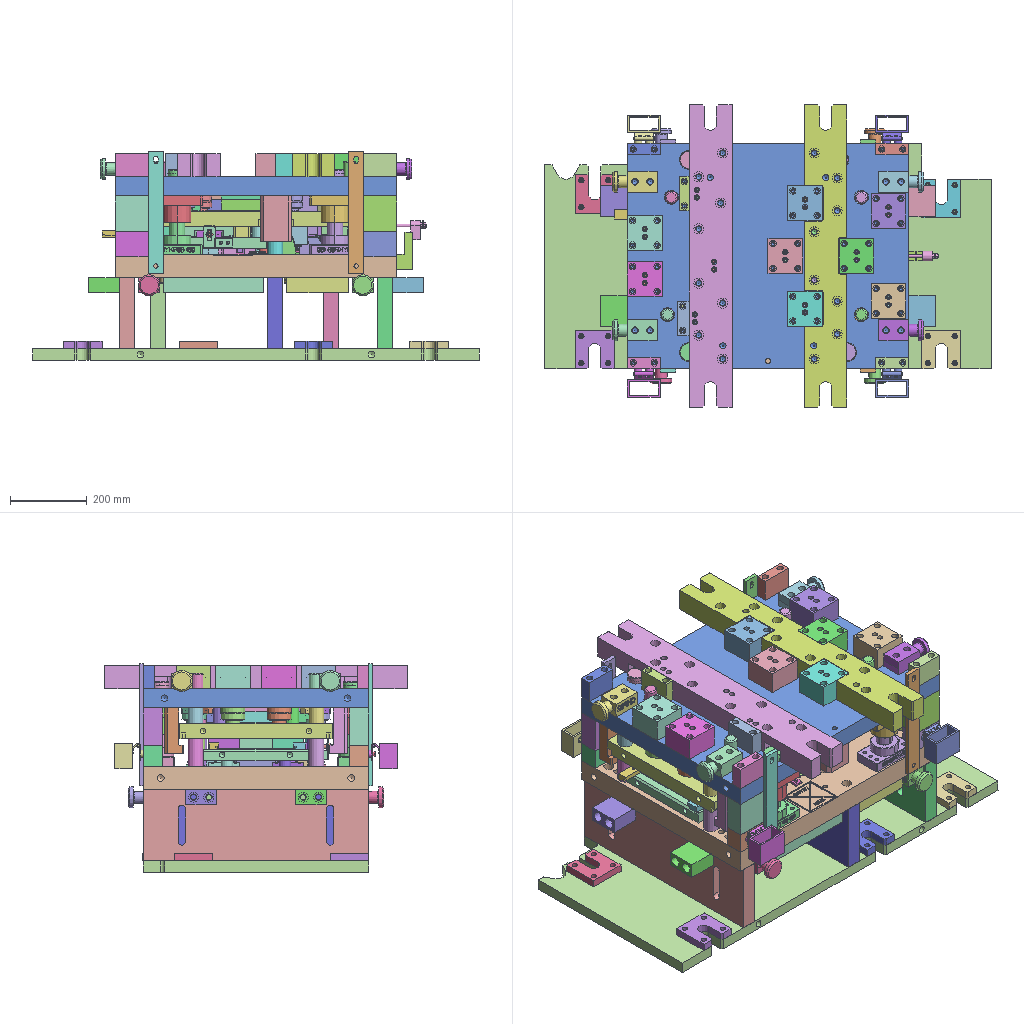Assembly | STEP file | 486 different items | 486 placed | box 1160 x 785 x 542 mm
Parts list (item | name | quantity | size | volume):
1 | 6-35_id1846_x_t | x1 | 8 x 8 x 38 mm | 1137 mm3
2 | 6-35_id1866_x_t | x1 | 8 x 8 x 38 mm | 1137 mm3
3 | - | x1 | 94 x 140 x 15 mm | 130830 mm3
4 | - | x1 | 58 x 85.001 x 56.5 mm | 200915 mm3
5 | - | x1 | 30 x 30 x 27 mm | 14276 mm3
6 | - | x1 | 30 x 30 x 27 mm | 14276 mm3
7 | - | x1 | 30 x 30 x 27 mm | 14276 mm3
8 | - | x1 | 60 x 80 x 56.5 mm | 99207 mm3
9 | - | x1 | 30 x 30 x 27 mm | 14276 mm3
10 | - | x1 | 40 x 40 x 72 mm | 79413 mm3
11 | - | x1 | 40 x 40 x 72 mm | 79413 mm3
12 | - | x1 | 40 x 40 x 72 mm | 79413 mm3
13 | - | x1 | 40 x 40 x 72 mm | 79413 mm3
14 | - | x1 | 99 x 140 x 30 mm | 280871 mm3
15 | - | x1 | 99 x 140 x 15 mm | 135777 mm3
16 | - | x1 | 40 x 40 x 72 mm | 79413 mm3
17 | - | x1 | 40 x 40 x 72 mm | 79413 mm3
18 | - | x1 | 42 x 25 x 98 mm | 60681 mm3
19 | - | x1 | 40 x 585 x 185 mm | 4078797 mm3
20 | - | x1 | 40 x 585 x 185 mm | 4012325 mm3
21 | - | x1 | 100 x 100 x 20 mm | 150755 mm3
22 | - | x1 | 100 x 100 x 20 mm | 150755 mm3
23 | - | x1 | 100 x 100 x 20 mm | 150755 mm3
24 | - | x1 | 40 x 255 x 185 mm | 1855337 mm3
25 | - | x1 | 40 x 255 x 185 mm | 1874377 mm3
26 | - | x1 | 40 x 585 x 185 mm | 4281820 mm3
27 | - | x1 | 85 x 50 x 55 mm | 210302 mm3
28 | - | x1 | 85 x 74 x 66.5 mm | 93814 mm3
29 | - | x1 | 63 x 73 x 30 mm | 93374 mm3
30 | - | x1 | 85 x 50 x 55 mm | 210302 mm3
31 | - | x1 | 85 x 74 x 66.5 mm | 93814 mm3
32 | - | x1 | 85 x 50 x 55 mm | 210302 mm3
33 | - | x1 | 85 x 74 x 66.5 mm | 93814 mm3
34 | - | x1 | 28 x 43 x 30 mm | 25680 mm3
35 | - | x1 | 85 x 50 x 55 mm | 210302 mm3
36 | - | x1 | 85 x 74 x 66.5 mm | 93814 mm3
37 | - | x1 | 19.1 x 19.1 x 30 mm | 8502 mm3
38 | - | x1 | 63 x 73 x 15 mm | 59595 mm3
39 | - | x1 | 30 x 30 x 15 mm | 8745 mm3
40 | - | x1 | 30 x 30 x 15 mm | 8745 mm3
41 | - | x1 | 30 x 30 x 15 mm | 8745 mm3
42 | - | x1 | 30 x 30 x 15 mm | 8745 mm3
43 | - | x1 | 30 x 30 x 15 mm | 8745 mm3
44 | - | x1 | 105 x 25 x 16 mm | 33608 mm3
45 | - | x1 | 45 x 25 x 16 mm | 13030 mm3
46 | - | x1 | 90 x 25 x 80 mm | 146448 mm3
47 | - | x1 | 90 x 25 x 80 mm | 146448 mm3
48 | - | x1 | 80 x 80 x 40 mm | 195367 mm3
49 | - | x1 | 80 x 80 x 40 mm | 195367 mm3
50 | - | x1 | 80 x 80 x 40 mm | 195367 mm3
51 | - | x1 | 80 x 80 x 40 mm | 195367 mm3
52 | - | x1 | 19.63 x 48.1 x 17 mm | 5552 mm3
53 | - | x1 | 75 x 27 x 53.7 mm | 8311 mm3
54 | - | x1 | 65 x 48 x 16 mm | 32002 mm3
55 | - | x1 | 15 x 70.5 x 16 mm | 11235 mm3
56 | - | x1 | 1160 x 585 x 30 mm | 18789042 mm3
57 | - | x1 | 100 x 100 x 20 mm | 150755 mm3
58 | - | x1 | 100 x 100 x 20 mm | 150755 mm3
59 | - | x1 | 260 x 40 x 40 mm | 385684 mm3
60 | - | x1 | - | 214873 mm3
61 | - | x1 | 260 x 40 x 40 mm | 385684 mm3
62 | - | x1 | 160 x 40 x 40 mm | 225684 mm3
63 | - | x1 | 160 x 40 x 40 mm | 225684 mm3
64 | - | x1 | 100 x 100 x 20 mm | 150755 mm3
65 | - | x1 | 40 x 10 x 317 mm | 124006 mm3
66 | - | x1 | 40 x 10 x 317 mm | 124006 mm3
67 | - | x1 | 40 x 10 x 317 mm | 124006 mm3
68 | - | x1 | 40 x 10 x 317 mm | 124006 mm3
69 | - | x1 | 58.148 x 85 x 56.5 mm | 200916 mm3
70 | - | x1 | 58 x 85 x 56.501 mm | 217515 mm3
71 | - | x1 | 40 x 55 x 53 mm | 73845 mm3
72 | - | x1 | 23.1 x 23.1 x 30 mm | 13334 mm3
73 | - | x1 | 65 x 75 x 45.001 mm | 106035 mm3
74 | - | x1 | 19 x 17 x 20 mm | 5075 mm3
75 | - | x1 | 15 x 13 x 20 mm | 2634 mm3
76 | - | x1 | 13.98 x 12 x 20 mm | 2357 mm3
77 | - | x1 | 70 x 120 x 30 mm | 188611 mm3
78 | - | x1 | 80 x 90 x 30 mm | 141495 mm3
79 | - | x1 | 80 x 90 x 15 mm | 69642 mm3
80 | - | x1 | 70 x 120 x 15 mm | 114867 mm3
81 | - | x1 | 40 x 55 x 53 mm | 73845 mm3
82 | - | x1 | 58 x 85 x 56.501 mm | 217785 mm3
83 | - | x1 | 58.914 x 80 x 15 mm | 42146 mm3
84 | - | x1 | 19.1 x 19.1 x 30 mm | 8502 mm3
85 | - | x1 | 60 x 80 x 56.5 mm | 99206 mm3
86 | - | x1 | 58.914 x 80 x 15 mm | 42146 mm3
87 | - | x1 | 105 x 25 x 16 mm | 33608 mm3
88 | - | x1 | 70 x 33 x 16 mm | 29565 mm3
89 | - | x1 | 20 x 25 x 7 mm | 3055 mm3
90 | - | x1 | 20 x 25 x 7 mm | 3055 mm3
91 | - | x1 | 20 x 25 x 7 mm | 3055 mm3
92 | - | x1 | 25 x 20 x 7 mm | 3055 mm3
93 | - | x1 | 730 x 585 x 60 mm | 23773121 mm3
94 | - | x1 | 240 x 52 x 30 mm | 250447 mm3
95 | - | x1 | 65 x 75 x 45.001 mm | 106042 mm3
96 | - | x1 | 19 x 17 x 20 mm | 5075 mm3
97 | - | x1 | 15 x 13 x 20 mm | 2634 mm3
98 | - | x1 | 13.98 x 12 x 20 mm | 2357 mm3
99 | - | x1 | 20 x 25 x 7 mm | 3055 mm3
100 | - | x1 | 26.045 x 93.231 x 17.45 mm | 4101 mm3
101 | - | x1 | 25 x 20 x 7 mm | 3055 mm3
102 | - | x1 | 94 x 140 x 30 mm | 271163 mm3
103 | - | x1 | 400 x 325 x 30 mm | 2323925 mm3
104 | CB-_id1534_x_t | x1 | 16 x 16 x 50 mm | 4584 mm3
105 | CB-_id1538_x_t | x1 | 16 x 16 x 50 mm | 4584 mm3
106 | CB-_id1554_x_t | x1 | 16 x 16 x 50 mm | 4584 mm3
107 | CB-_id1558_x_t | x1 | 16 x 16 x 50 mm | 4584 mm3
108 | CHP10_id1814_x_t | x1 | 118 x 55 x 55 mm | 202286 mm3
109 | CHP10_id1818_x_t | x1 | 118 x 55 x 55 mm | 202286 mm3
110 | CHP10_id1822_x_t | x1 | 118 x 55 x 55 mm | 202286 mm3
111 | CHP10_id1826_x_t | x1 | 118 x 55 x 55 mm | 202286 mm3
112 | CHP10_id1830_x_t | x1 | 55 x 118 x 55 mm | 202286 mm3
113 | CHP10_id1834_x_t | x1 | 55 x 118 x 55 mm | 202286 mm3
114 | CHP10_id1838_x_t | x1 | 55 x 118 x 55 mm | 202286 mm3
115 | CHP10_id1842_x_t | x1 | 55 x 118 x 55 mm | 202286 mm3
116 | D10-50_id1522_x_t | x1 | 10 x 10 x 50 mm | 3878 mm3
117 | D10-50_id1542_x_t | x1 | 10 x 10 x 50 mm | 3878 mm3
118 | D10-50_id1562_x_t | x1 | 10 x 10 x 50 mm | 3878 mm3
119 | D8-50_id106_x_t | x1 | 10 x 10 x 50 mm | 3919 mm3
120 | D8-50_id110_x_t | x1 | 10 x 10 x 50 mm | 3919 mm3
121 | D8-50_id114_x_t | x1 | 10 x 10 x 50 mm | 3919 mm3
122 | D8-50_id118_x_t | x1 | 10 x 10 x 50 mm | 3919 mm3
123 | D8-50_id1610_x_t | x1 | 8 x 8 x 30 mm | 1502 mm3
124 | D8-50_id1618_x_t | x1 | 8 x 8 x 30 mm | 1502 mm3
125 | D8-50_id162_x_t | x1 | 8 x 8 x 45 mm | 2256 mm3
126 | D8-50_id1630_x_t | x1 | 8 x 8 x 30 mm | 1502 mm3
127 | D8-50_id1638_x_t | x1 | 8 x 8 x 30 mm | 1502 mm3
128 | D8-50_id1650_x_t | x1 | 8 x 8 x 30 mm | 1502 mm3
129 | D8-50_id1654_x_t | x1 | 8 x 8 x 30 mm | 1502 mm3
130 | D8-50_id1658_x_t | x1 | 8 x 8 x 30 mm | 1502 mm3
131 | D8-50_id166_x_t | x1 | 8 x 8 x 45 mm | 2256 mm3
132 | D8-50_id1670_x_t | x1 | 8 x 8 x 30 mm | 1502 mm3
133 | D8-50_id1682_x_t | x1 | 8 x 8 x 30 mm | 1502 mm3
134 | D8-50_id1686_x_t | x1 | 8 x 8 x 30 mm | 1502 mm3
135 | D8-50_id290_x_t | x1 | 8 x 8 x 30 mm | 1502 mm3
136 | D8-50_id294_x_t | x1 | 8 x 8 x 30 mm | 1502 mm3
137 | D8-50_id350_x_t | x1 | 8 x 8 x 45 mm | 2256 mm3
138 | D8-50_id358_x_t | x1 | 8 x 8 x 45 mm | 2256 mm3
139 | D8-50_id390_x_t | x1 | 8 x 8 x 30 mm | 1502 mm3
140 | D8-50_id394_x_t | x1 | 8 x 8 x 30 mm | 1502 mm3
141 | D8-50_id402_x_t | x1 | 10 x 10 x 40 mm | 3134 mm3
142 | D8-50_id406_x_t | x1 | 8 x 8 x 30 mm | 1502 mm3
143 | D8-50_id422_x_t | x1 | 8 x 8 x 30 mm | 1502 mm3
144 | D8-50_id442_x_t | x1 | 10 x 10 x 40 mm | 3134 mm3
145 | D8-50_id470_x_t | x1 | 8 x 8 x 30 mm | 1502 mm3
146 | D8-50_id474_x_t | x1 | 8 x 8 x 30 mm | 1502 mm3
147 | D8-50_id482_x_t | x1 | 8 x 8 x 30 mm | 1502 mm3
148 | D8-50_id486_x_t | x1 | 8 x 8 x 30 mm | 1502 mm3
149 | D8-50_id50_x_t | x1 | 10 x 10 x 50 mm | 3919 mm3
150 | D8-50_id58_x_t | x1 | 10 x 10 x 50 mm | 3919 mm3
151 | D8-50_id618_x_t | x1 | 8 x 8 x 30 mm | 1502 mm3
152 | D8-50_id622_x_t | x1 | 8 x 8 x 30 mm | 1502 mm3
153 | D8-50_id78_x_t | x1 | 10 x 10 x 40 mm | 3134 mm3
154 | D8-50_id82_x_t | x1 | 10 x 10 x 40 mm | 3134 mm3
155 | GSV170-7_id1154_x_t | x1 | 50 x 50 x 114 mm | 158224 mm3
156 | GSV170-7_id1158_x_t | x1 | 50 x 50 x 114 mm | 158224 mm3
157 | GSV170-7_id1162_x_t | x1 | 50 x 50 x 114 mm | 158224 mm3
158 | GSV170-7_id1166_x_t | x1 | 50 x 50 x 114 mm | 158224 mm3
159 | GSV170-7_id1170_x_t | x1 | 50 x 50 x 114 mm | 158224 mm3
160 | GSV170-7_id1174_x_t | x1 | 50 x 50 x 114 mm | 158224 mm3
161 | GSV170-7_id1178_x_t | x1 | 63 x 63 x 120 mm | 273871 mm3
162 | GSV170-7_id1182_x_t | x1 | 63 x 63 x 120 mm | 273871 mm3
163 | GSV170-7_id1186_x_t | x1 | 63 x 63 x 120 mm | 273871 mm3
164 | GSV170-7_id1190_x_t | x1 | 63 x 63 x 120 mm | 273871 mm3
165 | GSV170-7_id1266_x_t | x1 | 50 x 50 x 114 mm | 158224 mm3
166 | GSV170-7_id502_x_t | x1 | 19 x 19 x 106 mm | 21365 mm3
167 | GSV170-7_id510_x_t | x1 | 19 x 19 x 106 mm | 21365 mm3
168 | GSV170-7_id526_x_t | x1 | 19 x 19 x 106 mm | 21365 mm3
169 | GSV170-7_id546_x_t | x1 | 19 x 19 x 106 mm | 21365 mm3
170 | GSV170-7_id666_x_t | x1 | 19 x 19 x 106 mm | 21365 mm3
171 | GSV170-7_id730_x_t | x1 | 19 x 19 x 106 mm | 21365 mm3
172 | LPS 2-10_id1006_x_t | x1 | 8 x 8 x 60 mm | 2567 mm3
173 | LPS 2-10_id1010_x_t | x1 | 8 x 8 x 60 mm | 2567 mm3
174 | LPS 2-10_id1014_x_t | x1 | 8 x 8 x 60 mm | 2567 mm3
175 | LPS 2-10_id1038_x_t | x1 | 8 x 8 x 60 mm | 2567 mm3
176 | LPS 2-10_id1042_x_t | x1 | 8 x 8 x 60 mm | 2567 mm3
177 | LPS 2-10_id1046_x_t | x1 | 8 x 8 x 60 mm | 2567 mm3
178 | LPS 2-10_id1050_x_t | x1 | 8 x 8 x 60 mm | 2567 mm3
179 | LPS 2-10_id898_x_t | x1 | 8 x 8 x 60 mm | 2567 mm3
180 | LPS 2-10_id902_x_t | x1 | 8 x 8 x 60 mm | 2567 mm3
181 | LPS 2-10_id906_x_t | x1 | 8 x 8 x 60 mm | 2567 mm3
182 | LPS 2-10_id910_x_t | x1 | 8 x 8 x 60 mm | 2567 mm3
183 | LPS 2-10_id914_x_t | x1 | 8 x 8 x 60 mm | 2567 mm3
184 | LPS 2-10_id918_x_t | x1 | 8 x 8 x 60 mm | 2567 mm3
185 | LPS 2-10_id922_x_t | x1 | 8 x 8 x 60 mm | 2567 mm3
186 | LPS 2-10_id926_x_t | x1 | 8 x 8 x 60 mm | 2567 mm3
187 | LPS 2-10_id930_x_t | x1 | 8 x 8 x 60 mm | 2567 mm3
188 | LPS 2-10_id934_x_t | x1 | 8 x 8 x 60 mm | 2567 mm3
189 | LPS 2-10_id938_x_t | x1 | 8 x 8 x 60 mm | 2567 mm3
190 | LPS 2-10_id942_x_t | x1 | 8 x 8 x 60 mm | 2567 mm3
191 | LPS 2-10_id946_x_t | x1 | 8 x 8 x 60 mm | 2567 mm3
192 | LPS 2-10_id950_x_t | x1 | 8 x 8 x 60 mm | 2567 mm3
193 | LPS 2-10_id954_x_t | x1 | 8 x 8 x 60 mm | 2567 mm3
194 | LPS 2-10_id974_x_t | x1 | 8 x 8 x 60 mm | 2567 mm3
195 | LPS 2-10_id978_x_t | x1 | 8 x 8 x 60 mm | 2567 mm3
196 | LPS 2-10_id982_x_t | x1 | 8 x 8 x 60 mm | 2567 mm3
197 | LPS 2-10_id986_x_t | x1 | 8 x 8 x 60 mm | 2567 mm3
198 | LPS 2-10_id990_x_t | x1 | 8 x 8 x 60 mm | 2567 mm3
199 | LPS 2-10_id994_x_t | x1 | 8 x 8 x 60 mm | 2567 mm3
200 | LPS 2-10_id998_x_t | x1 | 8 x 8 x 60 mm | 2567 mm3
201 | M3-10_id130_x_t | x1 | 16 x 16 x 55 mm | 4808 mm3
202 | M3-10_id134_x_t | x1 | 16 x 16 x 55 mm | 4808 mm3
203 | M3-10_id1366_x_t | x1 | 43 x 13 x 13 mm | 2482 mm3
204 | M3-10_id1414_x_t | x1 | 16 x 16 x 45 mm | 4022 mm3
205 | M3-10_id1418_x_t | x1 | 16 x 16 x 45 mm | 4022 mm3
206 | M3-10_id1422_x_t | x1 | 13 x 33 x 13 mm | 1987 mm3
207 | M3-10_id1426_x_t | x1 | 13 x 33 x 13 mm | 1987 mm3
208 | M3-10_id1434_x_t | x1 | 16 x 16 x 45 mm | 4022 mm3
209 | M3-10_id1438_x_t | x1 | 13 x 33 x 13 mm | 1987 mm3
210 | M3-10_id1442_x_t | x1 | 13 x 33 x 13 mm | 1987 mm3
211 | M3-10_id1454_x_t | x1 | 16 x 16 x 45 mm | 4022 mm3
212 | M3-10_id1474_x_t | x1 | 16 x 16 x 45 mm | 4022 mm3
213 | M3-10_id1486_x_t | x1 | 16 x 16 x 45 mm | 4022 mm3
214 | M3-10_id154_x_t | x1 | 13 x 13 x 48 mm | 2734 mm3
215 | M3-10_id1570_x_t | x1 | 13 x 13 x 28 mm | 1728 mm3
216 | M3-10_id1578_x_t | x1 | 13 x 13 x 28 mm | 1728 mm3
217 | M3-10_id1582_x_t | x1 | 13 x 13 x 28 mm | 1728 mm3
218 | M3-10_id158_x_t | x1 | 13 x 13 x 48 mm | 2734 mm3
219 | M3-10_id1594_x_t | x1 | 13 x 13 x 28 mm | 1728 mm3
220 | M3-10_id1602_x_t | x1 | 13 x 13 x 28 mm | 1728 mm3
221 | M3-10_id1614_x_t | x1 | 13 x 13 x 28 mm | 1742 mm3
222 | M3-10_id1622_x_t | x1 | 13 x 13 x 28 mm | 1742 mm3
223 | M3-10_id1634_x_t | x1 | 13 x 13 x 28 mm | 1742 mm3
224 | M3-10_id1646_x_t | x1 | 13 x 13 x 48 mm | 2734 mm3
225 | M3-10_id1662_x_t | x1 | 13 x 13 x 48 mm | 2734 mm3
226 | M3-10_id1674_x_t | x1 | 13 x 13 x 28 mm | 1742 mm3
227 | M3-10_id1678_x_t | x1 | 13 x 13 x 28 mm | 1742 mm3
228 | M3-10_id206_x_t | x1 | 20 x 8.5 x 8.5 mm | 482.387 mm3
229 | M3-10_id210_x_t | x1 | 20 x 8.5 x 8.5 mm | 482.387 mm3
230 | M3-10_id214_x_t | x1 | 16 x 16 x 40 mm | 3630 mm3
231 | M3-10_id218_x_t | x1 | 16 x 16 x 40 mm | 3630 mm3
232 | M3-10_id222_x_t | x1 | 16 x 16 x 40 mm | 3630 mm3
233 | M3-10_id226_x_t | x1 | 16 x 16 x 40 mm | 3630 mm3
234 | M3-10_id234_x_t | x1 | 16 x 16 x 40 mm | 3630 mm3
235 | M3-10_id238_x_t | x1 | 16 x 16 x 40 mm | 3630 mm3
236 | M3-10_id258_x_t | x1 | 8.5 x 8.5 x 20 mm | 456.375 mm3
237 | M3-10_id262_x_t | x1 | 8.5 x 8.5 x 20 mm | 456.375 mm3
238 | M3-10_id266_x_t | x1 | 8.5 x 8.5 x 20 mm | 456.375 mm3
239 | M3-10_id274_x_t | x1 | 10 x 10 x 46 mm | 1459 mm3
240 | M3-10_id278_x_t | x1 | 13 x 13 x 33 mm | 1980 mm3
241 | M3-10_id282_x_t | x1 | 13 x 13 x 33 mm | 1980 mm3
242 | M3-10_id286_x_t | x1 | 13 x 13 x 33 mm | 1980 mm3
243 | M3-10_id302_x_t | x1 | 20 x 8.5 x 8.5 mm | 482.387 mm3
244 | M3-10_id306_x_t | x1 | 16 x 16 x 40 mm | 3630 mm3
245 | M3-10_id310_x_t | x1 | 16 x 16 x 40 mm | 3630 mm3
246 | M3-10_id314_x_t | x1 | 20 x 8.5 x 8.5 mm | 482.387 mm3
247 | M3-10_id318_x_t | x1 | 16 x 16 x 40 mm | 3630 mm3
248 | M3-10_id322_x_t | x1 | 16 x 16 x 40 mm | 3630 mm3
249 | M3-10_id334_x_t | x1 | 16 x 16 x 40 mm | 3630 mm3
250 | M3-10_id342_x_t | x1 | 16 x 16 x 40 mm | 3630 mm3
251 | M3-10_id346_x_t | x1 | 13 x 13 x 48 mm | 2734 mm3
252 | M3-10_id34_x_t | x1 | 8.5 x 8.5 x 20 mm | 456.375 mm3
253 | M3-10_id354_x_t | x1 | 13 x 13 x 48 mm | 2734 mm3
254 | M3-10_id370_x_t | x1 | 8.5 x 8.5 x 20 mm | 456.375 mm3
255 | M3-10_id374_x_t | x1 | 13 x 13 x 28 mm | 1728 mm3
256 | M3-10_id378_x_t | x1 | 13 x 13 x 28 mm | 1728 mm3
257 | M3-10_id382_x_t | x1 | 13 x 13 x 28 mm | 1728 mm3
258 | M3-10_id386_x_t | x1 | 13 x 13 x 28 mm | 1728 mm3
259 | M3-10_id38_x_t | x1 | 8.5 x 8.5 x 20 mm | 456.375 mm3
260 | M3-10_id398_x_t | x1 | 13 x 13 x 28 mm | 1728 mm3
261 | M3-10_id410_x_t | x1 | 13 x 13 x 33 mm | 1980 mm3
262 | M3-10_id414_x_t | x1 | 13 x 13 x 33 mm | 1980 mm3
263 | M3-10_id418_x_t | x1 | 13 x 13 x 28 mm | 1728 mm3
264 | M3-10_id42_x_t | x1 | 16 x 16 x 55 mm | 4808 mm3
265 | M3-10_id430_x_t | x1 | 13 x 13 x 33 mm | 1980 mm3
266 | M3-10_id438_x_t | x1 | 13 x 13 x 28 mm | 1728 mm3
267 | M3-10_id446_x_t | x1 | 13 x 13 x 28 mm | 1728 mm3
268 | M3-10_id450_x_t | x1 | 13 x 13 x 33 mm | 1980 mm3
269 | M3-10_id462_x_t | x1 | 13 x 13 x 28 mm | 1742 mm3
270 | M3-10_id466_x_t | x1 | 13 x 13 x 28 mm | 1742 mm3
271 | M3-10_id46_x_t | x1 | 16 x 16 x 55 mm | 4808 mm3
272 | M3-10_id478_x_t | x1 | 13 x 13 x 28 mm | 1742 mm3
273 | M3-10_id54_x_t | x1 | 16 x 16 x 55 mm | 4808 mm3
274 | M3-10_id562_x_t | x1 | 10 x 10 x 26 mm | 877.848 mm3
275 | M3-10_id566_x_t | x1 | 10 x 10 x 26 mm | 877.848 mm3
276 | M3-10_id570_x_t | x1 | 10 x 10 x 26 mm | 877.848 mm3
277 | M3-10_id574_x_t | x1 | 10 x 10 x 26 mm | 877.848 mm3
278 | M3-10_id578_x_t | x1 | 10 x 10 x 26 mm | 877.848 mm3
279 | M3-10_id582_x_t | x1 | 10 x 10 x 26 mm | 877.848 mm3
280 | M3-10_id586_x_t | x1 | 10 x 10 x 26 mm | 877.848 mm3
281 | M3-10_id590_x_t | x1 | 10 x 10 x 26 mm | 877.848 mm3
282 | M3-10_id594_x_t | x1 | 13 x 13 x 28 mm | 1756 mm3
283 | M3-10_id598_x_t | x1 | 13 x 13 x 28 mm | 1756 mm3
284 | M3-10_id602_x_t | x1 | 13 x 13 x 28 mm | 1756 mm3
285 | M3-10_id610_x_t | x1 | 8.5 x 8.5 x 20 mm | 456.375 mm3
286 | M3-10_id626_x_t | x1 | 13 x 13 x 33 mm | 1980 mm3
287 | M3-10_id62_x_t | x1 | 13 x 13 x 33 mm | 1980 mm3
288 | M3-10_id630_x_t | x1 | 8.5 x 8.5 x 20 mm | 456.375 mm3
289 | M3-10_id634_x_t | x1 | 8.5 x 8.5 x 20 mm | 456.375 mm3
290 | M3-10_id642_x_t | x1 | 13 x 13 x 33 mm | 1980 mm3
291 | M3-10_id654_x_t | x1 | 13 x 13 x 33 mm | 1980 mm3
292 | M3-10_id658_x_t | x1 | 10 x 10 x 26 mm | 877.848 mm3
293 | M3-10_id662_x_t | x1 | 10 x 10 x 26 mm | 877.848 mm3
294 | M3-10_id66_x_t | x1 | 13 x 13 x 33 mm | 1980 mm3
295 | M3-10_id674_x_t | x1 | 13 x 13 x 33 mm | 1980 mm3
296 | M3-10_id678_x_t | x1 | 13 x 13 x 33 mm | 1980 mm3
297 | M3-10_id682_x_t | x1 | 13 x 13 x 33 mm | 1980 mm3
298 | M3-10_id686_x_t | x1 | 13 x 13 x 33 mm | 1980 mm3
299 | M3-10_id694_x_t | x1 | 13 x 13 x 33 mm | 1980 mm3
300 | M3-10_id702_x_t | x1 | 13 x 13 x 28 mm | 1756 mm3
301 | M3-10_id706_x_t | x1 | 10 x 10 x 26 mm | 877.848 mm3
302 | M3-10_id70_x_t | x1 | 13 x 13 x 33 mm | 1980 mm3
303 | M3-10_id710_x_t | x1 | 10 x 10 x 26 mm | 877.848 mm3
304 | M3-10_id714_x_t | x1 | 13 x 13 x 28 mm | 1756 mm3
305 | M3-10_id738_x_t | x1 | 13 x 13 x 33 mm | 1980 mm3
306 | M3-10_id74_x_t | x1 | 13 x 13 x 33 mm | 1980 mm3
307 | M3-10_id94_x_t | x1 | 16 x 16 x 55 mm | 4808 mm3
308 | M3-10_id98_x_t | x1 | 16 x 16 x 55 mm | 4808 mm3
309 | M6-40_id1082_x_t | x1 | 16 x 16 x 40 mm | 3648 mm3
310 | M6-40_id1090_x_t | x1 | 16 x 16 x 40 mm | 3648 mm3
311 | M6-40_id1098_x_t | x1 | 16 x 16 x 40 mm | 3648 mm3
312 | M6-40_id1106_x_t | x1 | 16 x 16 x 40 mm | 3648 mm3
313 | M6-40_id1114_x_t | x1 | 16 x 16 x 70 mm | 6004 mm3
314 | M6-40_id1122_x_t | x1 | 16 x 16 x 70 mm | 6004 mm3
315 | M6-40_id1126_x_t | x1 | 16 x 16 x 70 mm | 6004 mm3
316 | M6-40_id1130_x_t | x1 | 16 x 16 x 70 mm | 6004 mm3
317 | M6-40_id1138_x_t | x1 | 16 x 16 x 70 mm | 6004 mm3
318 | M6-40_id1146_x_t | x1 | 16 x 16 x 70 mm | 6004 mm3
319 | MSW12-10_id1850_x_t | x1 | 12.005 x 12.005 x 10 mm | 1118 mm3
320 | MSW12-10_id1862_x_t | x1 | 12.005 x 12.005 x 10 mm | 1118 mm3
321 | PN_0001_id1150_x_t | x1 | 730 x 585 x 50 mm | 18693036 mm3
322 | PN_0002_id1798_x_t | x1 | 85 x 30 x 60 mm | 133679 mm3
323 | PN_0002_id1802_x_t | x1 | 85 x 30 x 60 mm | 133679 mm3
324 | PN_0002_id1806_x_t | x1 | 85 x 30 x 60 mm | 133679 mm3
325 | PN_0002_id1810_x_t | x1 | 85 x 30 x 60 mm | 133679 mm3
326 | PN_0003_id1490_x_t | x1 | 90 x 90 x 60 mm | 430512 mm3
327 | PN_0003_id1494_x_t | x1 | 90 x 90 x 60 mm | 430512 mm3
328 | PN_0004_id1502_x_t | x1 | 30 x 90 x 60 mm | 142679 mm3
329 | PN_0005_id1498_x_t | x1 | 25 x 90 x 60 mm | 115679 mm3
330 | PN_0006_id1766_x_t | x1 | 112 x 785 x 60 mm | 4657225 mm3
331 | PN_0007_id1774_x_t | x1 | 90 x 90 x 60 mm | 428886 mm3
332 | PN_0007_id1778_x_t | x1 | 90 x 90 x 60 mm | 428886 mm3
333 | PN_0007_id1782_x_t | x1 | 90 x 90 x 60 mm | 428886 mm3
334 | PN_0007_id1786_x_t | x1 | 90 x 90 x 60 mm | 428886 mm3
335 | PN_0007_id1790_x_t | x1 | 90 x 90 x 60 mm | 428886 mm3
336 | PN_0007_id1794_x_t | x1 | 90 x 90 x 60 mm | 428886 mm3
337 | PN_0008_id1770_x_t | x1 | 110 x 785 x 60 mm | 3912002 mm3
338 | PN_0009_id1210_x_t | x1 | 40 x 40 x 40 mm | 44485 mm3
339 | PN_0009_id1214_x_t | x1 | 40 x 40 x 40 mm | 44485 mm3
340 | PN_0009_id1218_x_t | x1 | 40 x 40 x 40 mm | 44485 mm3
341 | PN_0009_id1222_x_t | x1 | 40 x 40 x 40 mm | 44485 mm3
342 | PN_0009_id1226_x_t | x1 | 40 x 40 x 40 mm | 44485 mm3
343 | PN_0009_id1230_x_t | x1 | 40 x 40 x 40 mm | 44485 mm3
344 | PN_0009_id1234_x_t | x1 | 40 x 40 x 40 mm | 44485 mm3
345 | PN_0009_id1238_x_t | x1 | 40 x 40 x 40 mm | 44485 mm3
346 | PN_0009_id1242_x_t | x1 | 40 x 40 x 40 mm | 44485 mm3
347 | PN_0009_id1246_x_t | x1 | 40 x 40 x 40 mm | 44485 mm3
348 | PN_0009_id1250_x_t | x1 | 40 x 40 x 40 mm | 44485 mm3
349 | PN_0009_id1254_x_t | x1 | 40 x 40 x 40 mm | 44485 mm3
350 | PN_0009_id1258_x_t | x1 | 40 x 40 x 40 mm | 44485 mm3
351 | PN_0009_id1262_x_t | x1 | 40 x 40 x 40 mm | 44485 mm3
352 | PN_0009_id1294_x_t | x1 | 40 x 40 x 40 mm | 44485 mm3
353 | PN_0009_id1302_x_t | x1 | 40 x 40 x 40 mm | 44485 mm3
354 | PN_0010_id1734_x_t | x1 | 30.406 x 30.406 x 15 mm | 5664 mm3
355 | PN_0010_id1738_x_t | x1 | 30.406 x 30.406 x 15 mm | 5664 mm3
356 | PN_0010_id1742_x_t | x1 | 28.807 x 23.857 x 15 mm | 5664 mm3
357 | PN_0010_id1746_x_t | x1 | 28.807 x 23.857 x 15 mm | 5664 mm3
358 | PN_0010_id1750_x_t | x1 | 27.746 x 22.068 x 15 mm | 5664 mm3
359 | PN_0010_id1754_x_t | x1 | 27.746 x 22.068 x 15 mm | 5664 mm3
360 | PN_0010_id1758_x_t | x1 | 29.858 x 30.721 x 15 mm | 5664 mm3
361 | PN_0010_id1762_x_t | x1 | 29.858 x 30.721 x 15 mm | 5664 mm3
362 | PN_0011_id1938_x_t | x1 | 30 x 16 x 16 mm | 6162 mm3
363 | PN_0012_id1934_x_t | x1 | 30 x 16 x 16 mm | 6162 mm3
364 | PN_0013_id878_x_t | x1 | 25 x 40 x 50 mm | 37635 mm3
365 | PN_0014_id874_x_t | x1 | 25 x 40 x 50 mm | 37635 mm3
366 | PN_0015_id866_x_t | x1 | 95 x 130 x 28 mm | 241686 mm3
367 | PN_0016_id882_x_t | x1 | 40 x 25 x 50 mm | 37460 mm3
368 | PN_0017_id886_x_t | x1 | 90 x 75 x 28 mm | 120807 mm3
369 | PN_0018_id894_x_t | x1 | 43 x 30 x 50 mm | 41594 mm3
370 | PN_0019_id962_x_t | x1 | 105 x 120 x 28 mm | 217134 mm3
371 | PN_0020_id958_x_t | x1 | 105 x 120 x 28 mm | 217134 mm3
372 | PN_0021_id1034_x_t | x1 | 51 x 55 x 50 mm | 79399 mm3
373 | PN_0022_id1018_x_t | x1 | 105 x 176 x 28 mm | 281247 mm3
374 | PN_0023_id1002_x_t | x1 | 51 x 55 x 50 mm | 79567 mm3
375 | PN_0024_id1030_x_t | x1 | 60 x 85 x 28 mm | 85179 mm3
376 | PN_0025_id842_x_t | x1 | 727.5 x 395 x 40 mm | 9281090 mm3
377 | PN_0026_id138_x_t | x1 | 15 x 17 x 108 mm | 21787 mm3
378 | PN_0027_id762_x_t | x1 | 48.641 x 98 x 108 mm | 278629 mm3
379 | PN_0028_id758_x_t | x1 | 48.641 x 98 x 108 mm | 278628 mm3
380 | PN_0029_id850_x_t | x1 | 51.676 x 85.003 x 65 mm | 145640 mm3
381 | PN_0030_id186_x_t | x1 | 51.676 x 85 x 65 mm | 145641 mm3
382 | PN_0031_id862_x_t | x1 | 42.5 x 42 x 101 mm | 91343 mm3
383 | PN_0032_id1054_x_t | x1 | 63.914 x 80 x 35 mm | 137778 mm3
384 | PN_0033_id754_x_t | x1 | 63.914 x 80 x 35 mm | 137778 mm3
385 | PN_0034_id750_x_t | x1 | 290 x 208 x 25 mm | 1200557 mm3
386 | PN_0035_id190_x_t | x1 | 50.466 x 210 x 37 mm | 295873 mm3
387 | PN_0036_id230_x_t | x1 | 149.23 x 42 x 25 mm | 138214 mm3
388 | PN_0037_id1074_x_t | x1 | 70 x 85 x 53 mm | 208410 mm3
389 | PN_0038_id1942_x_t | x1 | 70 x 85 x 53 mm | 208411 mm3
390 | PN_0039_id846_x_t | x1 | 115 x 175 x 25 mm | 409284 mm3
391 | PN_0040_id1406_x_t | x1 | 85 x 50 x 97 mm | 372174 mm3
392 | PN_0040_id1446_x_t | x1 | 85 x 50 x 97 mm | 372174 mm3
393 | PN_0040_id1462_x_t | x1 | 85 x 50 x 97 mm | 372174 mm3
394 | PN_0040_id1478_x_t | x1 | 85 x 50 x 97 mm | 372174 mm3
395 | PN_0041_id1270_x_t | x1 | 80 x 50 x 118 mm | 264145 mm3
396 | PN_0041_id1274_x_t | x1 | 80 x 50 x 118 mm | 264145 mm3
397 | PN_0041_id1278_x_t | x1 | 80 x 50 x 118 mm | 264145 mm3
398 | PN_0041_id1282_x_t | x1 | 80 x 50 x 118 mm | 264145 mm3
399 | PN_0041_id1286_x_t | x1 | 80 x 50 x 118 mm | 264145 mm3
400 | PN_0041_id1290_x_t | x1 | 80 x 50 x 118 mm | 264145 mm3
401 | PN_0042_id870_x_t | x1 | 95 x 130 x 10 mm | 115889 mm3
402 | PN_0043_id890_x_t | x1 | 90 x 75 x 10 mm | 57234 mm3
403 | PN_0044_id966_x_t | x1 | 105 x 120 x 10 mm | 118397 mm3
404 | PN_0044_id970_x_t | x1 | 105 x 120 x 10 mm | 118397 mm3
405 | PN_0045_id858_x_t | x1 | 74.676 x 85 x 110 mm | 490058 mm3
406 | PN_0046_id854_x_t | x1 | 74.676 x 85 x 110 mm | 490062 mm3
407 | PN_0047_id1022_x_t | x1 | 105 x 176 x 10 mm | 142706 mm3
408 | PN_0048_id1026_x_t | x1 | 60 x 85 x 10 mm | 42512 mm3
409 | PN_0049_id1058_x_t | x1 | 13 x 13 x 100 mm | 5213 mm3
410 | PN_0049_id1062_x_t | x1 | 13 x 13 x 100 mm | 5213 mm3
411 | PN_0050_id1066_x_t | x1 | 15 x 15 x 100 mm | 8031 mm3
412 | PN_0051_id1710_x_t | x1 | 13 x 13 x 100 mm | 4994 mm3
413 | PN_0051_id1714_x_t | x1 | 13 x 13 x 100 mm | 4994 mm3
414 | PN_0052_id1718_x_t | x1 | 15 x 15 x 100 mm | 7737 mm3
415 | PN_0052_id1722_x_t | x1 | 15 x 15 x 100 mm | 7737 mm3
416 | PN_0053_id1726_x_t | x1 | 15 x 11.5 x 100 mm | 7176 mm3
417 | PN_0053_id1730_x_t | x1 | 15 x 11.5 x 100 mm | 7176 mm3
418 | PN_0054_id498_x_t | x1 | 45 x 25 x 9.2 mm | 6185 mm3
419 | PN_0054_id518_x_t | x1 | 45 x 25 x 9.2 mm | 6185 mm3
420 | PN_0054_id534_x_t | x1 | 45 x 25 x 9.2 mm | 6185 mm3
421 | PN_0054_id554_x_t | x1 | 45 x 25 x 9.2 mm | 6185 mm3
422 | PN_0054_id670_x_t | x1 | 25 x 45 x 9.2 mm | 6185 mm3
423 | PN_0054_id722_x_t | x1 | 25 x 45 x 9.2 mm | 6185 mm3
424 | PN_0055_id1202_x_t | x1 | 42 x 42 x 40 mm | 22994 mm3
425 | PN_0055_id1322_x_t | x1 | 42 x 42 x 40 mm | 22995 mm3
426 | PN_0055_id1330_x_t | x1 | 42 x 42 x 40 mm | 22994 mm3
427 | PN_0055_id1354_x_t | x1 | 42 x 42 x 40 mm | 22995 mm3
428 | PN_0056_id1706_x_t | x1 | 16 x 16 x 45 mm | 3853 mm3
429 | PN_0057_id1194_x_t | x1 | 44 x 44 x 153 mm | 127630 mm3
430 | PN_0057_id1198_x_t | x1 | 16 x 16 x 40 mm | 4064 mm3
431 | PN_0057_id1206_x_t | x1 | 40 x 40 x 16 mm | 13382 mm3
432 | PN_0057_id1310_x_t | x1 | 44 x 44 x 153 mm | 127629 mm3
433 | PN_0057_id1314_x_t | x1 | 40 x 40 x 16 mm | 13382 mm3
434 | PN_0057_id1318_x_t | x1 | 16 x 16 x 40 mm | 4064 mm3
435 | PN_0057_id1326_x_t | x1 | 44 x 44 x 153 mm | 127630 mm3
436 | PN_0057_id1334_x_t | x1 | 40 x 40 x 16 mm | 13382 mm3
437 | PN_0057_id1338_x_t | x1 | 16 x 16 x 40 mm | 4064 mm3
438 | PN_0057_id1342_x_t | x1 | 16 x 16 x 40 mm | 4064 mm3
439 | PN_0057_id1346_x_t | x1 | 44 x 44 x 153 mm | 127629 mm3
440 | PN_0057_id1350_x_t | x1 | 40 x 40 x 16 mm | 13382 mm3
441 | PN_0058_id1506_x_t | x1 | 130 x 75 x 70 mm | 291088 mm3
442 | PN_0058_id1510_x_t | x1 | 130 x 75 x 220 mm | 598119 mm3
443 | PN_0058_id1514_x_t | x1 | 130 x 75 x 220 mm | 598119 mm3
444 | PN_0058_id1518_x_t | x1 | 130 x 75 x 70 mm | 291088 mm3
445 | PN_0058_id1526_x_t | x1 | 130 x 75 x 220 mm | 598119 mm3
446 | PN_0058_id1530_x_t | x1 | 130 x 75 x 70 mm | 291088 mm3
447 | PN_0058_id1546_x_t | x1 | 130 x 75 x 220 mm | 598119 mm3
448 | PN_0058_id1550_x_t | x1 | 130 x 75 x 70 mm | 291088 mm3
449 | PN_0059_id1358_x_t | x1 | 86 x 30 x 52 mm | 33398 mm3
450 | PN_0060_id538_x_t | x1 | 20 x 20 x 100 mm | 28952 mm3
451 | PN_0060_id734_x_t | x1 | 20 x 20 x 100 mm | 28953 mm3
452 | PN_0061_id1870_x_t | x1 | 20 x 20 x 100 mm | 29183 mm3
453 | PN_0061_id1874_x_t | x1 | 20 x 20 x 100 mm | 29183 mm3
454 | PN_0061_id1878_x_t | x1 | 20 x 20 x 100 mm | 29183 mm3
455 | PN_0061_id1882_x_t | x1 | 20 x 20 x 100 mm | 29183 mm3
456 | PN_0062_id766_x_t | x1 | 9 x 9 x 33.641 mm | 968.209 mm3
457 | PN_0062_id770_x_t | x1 | 9 x 9 x 33.641 mm | 968.209 mm3
458 | PN_0062_id774_x_t | x1 | 9 x 9 x 33.641 mm | 968.209 mm3
459 | PN_0062_id778_x_t | x1 | 9 x 9 x 33.641 mm | 968.209 mm3
460 | PN_0062_id782_x_t | x1 | 9 x 9 x 33.641 mm | 968.209 mm3
461 | PN_0062_id786_x_t | x1 | 9 x 9 x 33.641 mm | 968.209 mm3
462 | PN_0063_id790_x_t | x1 | 11 x 11 x 34.5 mm | 1696 mm3
463 | PN_0063_id794_x_t | x1 | 11 x 11 x 34.5 mm | 1696 mm3
464 | PN_0063_id798_x_t | x1 | 11 x 11 x 34.5 mm | 1696 mm3
465 | PN_0063_id802_x_t | x1 | 11 x 11 x 34.5 mm | 1696 mm3
466 | PN_0063_id806_x_t | x1 | 11 x 11 x 34.5 mm | 1696 mm3
467 | PN_0063_id810_x_t | x1 | 11 x 11 x 34.5 mm | 1696 mm3
468 | PN_0063_id814_x_t | x1 | 11 x 11 x 34.5 mm | 1696 mm3
469 | PN_0063_id818_x_t | x1 | 11 x 11 x 34.5 mm | 1696 mm3
470 | PN_0063_id822_x_t | x1 | 11 x 11 x 34.5 mm | 1696 mm3
471 | PN_0063_id826_x_t | x1 | 11 x 11 x 34.5 mm | 1696 mm3
472 | PN_0063_id830_x_t | x1 | 11 x 11 x 34.5 mm | 1696 mm3
473 | PN_0063_id834_x_t | x1 | 11 x 11 x 34.5 mm | 1696 mm3
474 | PN_0063_id838_x_t | x1 | 11 x 11 x 34.5 mm | 1696 mm3
475 | PN_0064_id202_x_t | x1 | 10.01 x 50 x 22 mm | 9849 mm3
476 | PN_0064_id326_x_t | x1 | 10.01 x 50 x 22 mm | 9849 mm3
477 | SGBH 20-16_id490_x_t | x1 | 28 x 28 x 35 mm | 6555 mm3
478 | SGBH 20-16_id506_x_t | x1 | 28 x 28 x 35 mm | 6555 mm3
479 | SGBH 20-16_id522_x_t | x1 | 28 x 28 x 35 mm | 6555 mm3
480 | SGBH 20-16_id542_x_t | x1 | 28 x 28 x 35 mm | 6555 mm3
481 | SGBH 20-16_id690_x_t | x1 | 28 x 28 x 35 mm | 6555 mm3
482 | SGBH 20-16_id726_x_t | x1 | 28 x 28 x 35 mm | 6555 mm3
483 | SWF10-15_id1854_x_t | x1 | 10 x 10 x 55 mm | 2723 mm3
484 | SWF10-15_id1858_x_t | x1 | 10 x 10 x 55 mm | 2723 mm3
485 | SWF8-30_id742_x_t | x1 | 12 x 12 x 70 mm | 4273 mm3
486 | SWM_id746_x_t | x1 | 16 x 16 x 10 mm | 1720 mm3